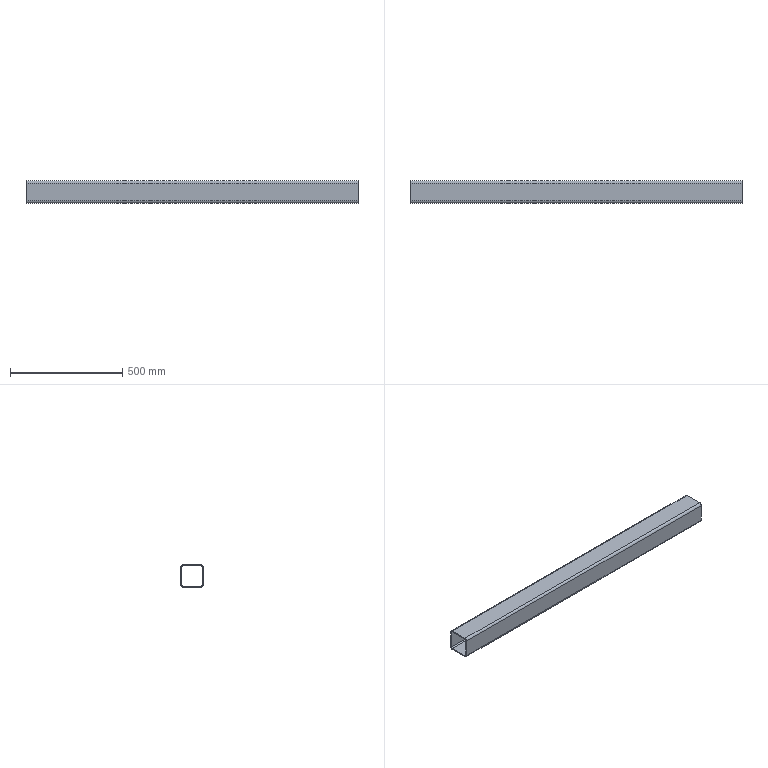Part | SolidWorks | features BaseBody 1 | 1 solid | 18 faces | box 1480 x 100 x 100 mm | volume 2716717 mm3 | plane 10 | cylinder 8 | commonest cylinder face diameters 10 x4 20 x4
STEP:
#1=CARTESIAN_POINT('',(-740.,40.,-50.));
#2=VERTEX_POINT('',#1);
#3=CARTESIAN_POINT('',(-740.,50.,-40.));
#4=VERTEX_POINT('',#3);
#5=CARTESIAN_POINT('',(-740.,40.,-40.));
#6=DIRECTION('',(1.,0.,0.));
#7=DIRECTION('',(0.,0.,-1.));
#8=AXIS2_PLACEMENT_3D('',#5,#6,#7);
#9=CIRCLE('',#8,10.);
#10=EDGE_CURVE('',#2,#4,#9,.T.);
#11=ORIENTED_EDGE('',*,*,#10,.T.);
#12=CARTESIAN_POINT('',(740.,50.,-40.));
#13=VERTEX_POINT('',#12);
#14=CARTESIAN_POINT('',(740.,50.,-40.));
#15=DIRECTION('',(-1.,0.,0.));
#16=VECTOR('',#15,1000.);
#17=LINE('',#14,#16);
#18=EDGE_CURVE('',#13,#4,#17,.T.);
#19=ORIENTED_EDGE('',*,*,#18,.F.);
#20=CARTESIAN_POINT('',(740.,40.,-50.));
#21=VERTEX_POINT('',#20);
#22=CARTESIAN_POINT('',(740.,40.,-40.));
#23=DIRECTION('',(1.,0.,0.));
#24=DIRECTION('',(0.,0.,-1.));
#25=AXIS2_PLACEMENT_3D('',#22,#23,#24);
#26=CIRCLE('',#25,10.);
#27=EDGE_CURVE('',#21,#13,#26,.T.);
#28=ORIENTED_EDGE('',*,*,#27,.F.);
#29=CARTESIAN_POINT('',(740.,40.,-50.));
#30=DIRECTION('',(-1.,0.,0.));
#31=VECTOR('',#30,1000.);
#32=LINE('',#29,#31);
#33=EDGE_CURVE('',#21,#2,#32,.T.);
#34=ORIENTED_EDGE('',*,*,#33,.T.);
#35=EDGE_LOOP('',(#11,#19,#28,#34));
#36=FACE_OUTER_BOUND('',#35,.T.);
#37=CARTESIAN_POINT('',(740.,40.,-40.));
#38=DIRECTION('',(-1.,0.,0.));
#39=DIRECTION('',(0.,0.,1.));
#40=AXIS2_PLACEMENT_3D('',#37,#38,#39);
#41=CYLINDRICAL_SURFACE('',#40,10.);
#42=ADVANCED_FACE('',(#36),#41,.T.);
#43=CARTESIAN_POINT('',(-740.,50.,40.));
#44=VERTEX_POINT('',#43);
#45=CARTESIAN_POINT('',(-740.,50.,-40.));
#46=DIRECTION('',(0.,0.,1.));
#47=VECTOR('',#46,1000.);
#48=LINE('',#45,#47);
#49=EDGE_CURVE('',#4,#44,#48,.T.);
#50=ORIENTED_EDGE('',*,*,#49,.T.);
#51=CARTESIAN_POINT('',(740.,50.,40.));
#52=VERTEX_POINT('',#51);
#53=CARTESIAN_POINT('',(740.,50.,40.));
#54=DIRECTION('',(-1.,0.,0.));
#55=VECTOR('',#54,1000.);
#56=LINE('',#53,#55);
#57=EDGE_CURVE('',#52,#44,#56,.T.);
#58=ORIENTED_EDGE('',*,*,#57,.F.);
#59=CARTESIAN_POINT('',(740.,50.,-40.));
#60=DIRECTION('',(0.,0.,1.));
#61=VECTOR('',#60,1000.);
#62=LINE('',#59,#61);
#63=EDGE_CURVE('',#13,#52,#62,.T.);
#64=ORIENTED_EDGE('',*,*,#63,.F.);
#65=ORIENTED_EDGE('',*,*,#18,.T.);
#66=EDGE_LOOP('',(#50,#58,#64,#65));
#67=FACE_OUTER_BOUND('',#66,.T.);
#68=CARTESIAN_POINT('',(740.,50.,-40.));
#69=DIRECTION('',(0.,-1.,0.));
#70=DIRECTION('',(0.,0.,-1.));
#71=AXIS2_PLACEMENT_3D('',#68,#69,#70);
#72=PLANE('',#71);
#73=ADVANCED_FACE('',(#67),#72,.F.);
#74=CARTESIAN_POINT('',(-740.,40.,50.));
#75=VERTEX_POINT('',#74);
#76=CARTESIAN_POINT('',(-740.,40.,40.));
#77=DIRECTION('',(1.,0.,0.));
#78=DIRECTION('',(0.,0.,-1.));
#79=AXIS2_PLACEMENT_3D('',#76,#77,#78);
#80=CIRCLE('',#79,10.);
#81=EDGE_CURVE('',#44,#75,#80,.T.);
#82=ORIENTED_EDGE('',*,*,#81,.T.);
#83=CARTESIAN_POINT('',(740.,40.,50.));
#84=VERTEX_POINT('',#83);
#85=CARTESIAN_POINT('',(740.,40.,50.));
#86=DIRECTION('',(-1.,0.,0.));
#87=VECTOR('',#86,1000.);
#88=LINE('',#85,#87);
#89=EDGE_CURVE('',#84,#75,#88,.T.);
#90=ORIENTED_EDGE('',*,*,#89,.F.);
#91=CARTESIAN_POINT('',(740.,40.,40.));
#92=DIRECTION('',(1.,0.,0.));
#93=DIRECTION('',(0.,0.,-1.));
#94=AXIS2_PLACEMENT_3D('',#91,#92,#93);
#95=CIRCLE('',#94,10.);
#96=EDGE_CURVE('',#52,#84,#95,.T.);
#97=ORIENTED_EDGE('',*,*,#96,.F.);
#98=ORIENTED_EDGE('',*,*,#57,.T.);
#99=EDGE_LOOP('',(#82,#90,#97,#98));
#100=FACE_OUTER_BOUND('',#99,.T.);
#101=CARTESIAN_POINT('',(740.,40.,40.));
#102=DIRECTION('',(-1.,0.,0.));
#103=DIRECTION('',(0.,0.,1.));
#104=AXIS2_PLACEMENT_3D('',#101,#102,#103);
#105=CYLINDRICAL_SURFACE('',#104,10.);
#106=ADVANCED_FACE('',(#100),#105,.T.);
#107=CARTESIAN_POINT('',(-740.,-40.,50.));
#108=VERTEX_POINT('',#107);
#109=CARTESIAN_POINT('',(-740.,-40.,50.));
#110=DIRECTION('',(0.,-1.,0.));
#111=VECTOR('',#110,1000.);
#112=LINE('',#109,#111);
#113=EDGE_CURVE('',#75,#108,#112,.T.);
#114=ORIENTED_EDGE('',*,*,#113,.T.);
#115=CARTESIAN_POINT('',(740.,-40.,50.));
#116=VERTEX_POINT('',#115);
#117=CARTESIAN_POINT('',(740.,-40.,50.));
#118=DIRECTION('',(-1.,0.,0.));
#119=VECTOR('',#118,1000.);
#120=LINE('',#117,#119);
#121=EDGE_CURVE('',#116,#108,#120,.T.);
#122=ORIENTED_EDGE('',*,*,#121,.F.);
#123=CARTESIAN_POINT('',(740.,-40.,50.));
#124=DIRECTION('',(0.,-1.,0.));
#125=VECTOR('',#124,1000.);
#126=LINE('',#123,#125);
#127=EDGE_CURVE('',#84,#116,#126,.T.);
#128=ORIENTED_EDGE('',*,*,#127,.F.);
#129=ORIENTED_EDGE('',*,*,#89,.T.);
#130=EDGE_LOOP('',(#114,#122,#128,#129));
#131=FACE_OUTER_BOUND('',#130,.T.);
#132=CARTESIAN_POINT('',(740.,-40.,50.));
#133=DIRECTION('',(0.,0.,-1.));
#134=DIRECTION('',(-1.,0.,0.));
#135=AXIS2_PLACEMENT_3D('',#132,#133,#134);
#136=PLANE('',#135);
#137=ADVANCED_FACE('',(#131),#136,.F.);
#138=CARTESIAN_POINT('',(-740.,-50.,40.));
#139=VERTEX_POINT('',#138);
#140=CARTESIAN_POINT('',(-740.,-40.,40.));
#141=DIRECTION('',(1.,0.,0.));
#142=DIRECTION('',(0.,0.,-1.));
#143=AXIS2_PLACEMENT_3D('',#140,#141,#142);
#144=CIRCLE('',#143,10.);
#145=EDGE_CURVE('',#108,#139,#144,.T.);
#146=ORIENTED_EDGE('',*,*,#145,.T.);
#147=CARTESIAN_POINT('',(740.,-50.,40.));
#148=VERTEX_POINT('',#147);
#149=CARTESIAN_POINT('',(740.,-50.,40.));
#150=DIRECTION('',(-1.,0.,0.));
#151=VECTOR('',#150,1000.);
#152=LINE('',#149,#151);
#153=EDGE_CURVE('',#148,#139,#152,.T.);
#154=ORIENTED_EDGE('',*,*,#153,.F.);
#155=CARTESIAN_POINT('',(740.,-40.,40.));
#156=DIRECTION('',(1.,0.,0.));
#157=DIRECTION('',(0.,0.,-1.));
#158=AXIS2_PLACEMENT_3D('',#155,#156,#157);
#159=CIRCLE('',#158,10.);
#160=EDGE_CURVE('',#116,#148,#159,.T.);
#161=ORIENTED_EDGE('',*,*,#160,.F.);
#162=ORIENTED_EDGE('',*,*,#121,.T.);
#163=EDGE_LOOP('',(#146,#154,#161,#162));
#164=FACE_OUTER_BOUND('',#163,.T.);
#165=CARTESIAN_POINT('',(740.,-40.,40.));
#166=DIRECTION('',(-1.,0.,0.));
#167=DIRECTION('',(0.,0.,1.));
#168=AXIS2_PLACEMENT_3D('',#165,#166,#167);
#169=CYLINDRICAL_SURFACE('',#168,10.);
#170=ADVANCED_FACE('',(#164),#169,.T.);
#171=CARTESIAN_POINT('',(-740.,-50.,-40.));
#172=VERTEX_POINT('',#171);
#173=CARTESIAN_POINT('',(-740.,-50.,40.));
#174=DIRECTION('',(0.,0.,-1.));
#175=VECTOR('',#174,1000.);
#176=LINE('',#173,#175);
#177=EDGE_CURVE('',#139,#172,#176,.T.);
#178=ORIENTED_EDGE('',*,*,#177,.T.);
#179=CARTESIAN_POINT('',(740.,-50.,-40.));
#180=VERTEX_POINT('',#179);
#181=CARTESIAN_POINT('',(740.,-50.,-40.));
#182=DIRECTION('',(-1.,0.,0.));
#183=VECTOR('',#182,1000.);
#184=LINE('',#181,#183);
#185=EDGE_CURVE('',#180,#172,#184,.T.);
#186=ORIENTED_EDGE('',*,*,#185,.F.);
#187=CARTESIAN_POINT('',(740.,-50.,40.));
#188=DIRECTION('',(0.,0.,-1.));
#189=VECTOR('',#188,1000.);
#190=LINE('',#187,#189);
#191=EDGE_CURVE('',#148,#180,#190,.T.);
#192=ORIENTED_EDGE('',*,*,#191,.F.);
#193=ORIENTED_EDGE('',*,*,#153,.T.);
#194=EDGE_LOOP('',(#178,#186,#192,#193));
#195=FACE_OUTER_BOUND('',#194,.T.);
#196=CARTESIAN_POINT('',(740.,-50.,40.));
#197=DIRECTION('',(0.,1.,0.));
#198=DIRECTION('',(0.,0.,1.));
#199=AXIS2_PLACEMENT_3D('',#196,#197,#198);
#200=PLANE('',#199);
#201=ADVANCED_FACE('',(#195),#200,.F.);
#202=CARTESIAN_POINT('',(-740.,-40.,-50.));
#203=VERTEX_POINT('',#202);
#204=CARTESIAN_POINT('',(-740.,-40.,-40.));
#205=DIRECTION('',(1.,0.,0.));
#206=DIRECTION('',(0.,0.,-1.));
#207=AXIS2_PLACEMENT_3D('',#204,#205,#206);
#208=CIRCLE('',#207,10.);
#209=EDGE_CURVE('',#172,#203,#208,.T.);
#210=ORIENTED_EDGE('',*,*,#209,.T.);
#211=CARTESIAN_POINT('',(740.,-40.,-50.));
#212=VERTEX_POINT('',#211);
#213=CARTESIAN_POINT('',(740.,-40.,-50.));
#214=DIRECTION('',(-1.,0.,0.));
#215=VECTOR('',#214,1000.);
#216=LINE('',#213,#215);
#217=EDGE_CURVE('',#212,#203,#216,.T.);
#218=ORIENTED_EDGE('',*,*,#217,.F.);
#219=CARTESIAN_POINT('',(740.,-40.,-40.));
#220=DIRECTION('',(1.,0.,0.));
#221=DIRECTION('',(0.,0.,-1.));
#222=AXIS2_PLACEMENT_3D('',#219,#220,#221);
#223=CIRCLE('',#222,10.);
#224=EDGE_CURVE('',#180,#212,#223,.T.);
#225=ORIENTED_EDGE('',*,*,#224,.F.);
#226=ORIENTED_EDGE('',*,*,#185,.T.);
#227=EDGE_LOOP('',(#210,#218,#225,#226));
#228=FACE_OUTER_BOUND('',#227,.T.);
#229=CARTESIAN_POINT('',(740.,-40.,-40.));
#230=DIRECTION('',(-1.,0.,0.));
#231=DIRECTION('',(0.,0.,1.));
#232=AXIS2_PLACEMENT_3D('',#229,#230,#231);
#233=CYLINDRICAL_SURFACE('',#232,10.);
#234=ADVANCED_FACE('',(#228),#233,.T.);
#235=CARTESIAN_POINT('',(-740.,45.,40.));
#236=VERTEX_POINT('',#235);
#237=CARTESIAN_POINT('',(-740.,40.,45.));
#238=VERTEX_POINT('',#237);
#239=CARTESIAN_POINT('',(-740.,40.,40.));
#240=DIRECTION('',(1.,0.,0.));
#241=DIRECTION('',(0.,0.,-1.));
#242=AXIS2_PLACEMENT_3D('',#239,#240,#241);
#243=CIRCLE('',#242,5.);
#244=EDGE_CURVE('',#236,#238,#243,.T.);
#245=ORIENTED_EDGE('',*,*,#244,.F.);
#246=CARTESIAN_POINT('',(740.,45.,40.));
#247=VERTEX_POINT('',#246);
#248=CARTESIAN_POINT('',(740.,45.,40.));
#249=DIRECTION('',(-1.,0.,0.));
#250=VECTOR('',#249,1000.);
#251=LINE('',#248,#250);
#252=EDGE_CURVE('',#247,#236,#251,.T.);
#253=ORIENTED_EDGE('',*,*,#252,.F.);
#254=CARTESIAN_POINT('',(740.,40.,45.));
#255=VERTEX_POINT('',#254);
#256=CARTESIAN_POINT('',(740.,40.,40.));
#257=DIRECTION('',(1.,0.,0.));
#258=DIRECTION('',(0.,0.,-1.));
#259=AXIS2_PLACEMENT_3D('',#256,#257,#258);
#260=CIRCLE('',#259,5.);
#261=EDGE_CURVE('',#247,#255,#260,.T.);
#262=ORIENTED_EDGE('',*,*,#261,.T.);
#263=CARTESIAN_POINT('',(740.,40.,45.));
#264=DIRECTION('',(-1.,0.,0.));
#265=VECTOR('',#264,1000.);
#266=LINE('',#263,#265);
#267=EDGE_CURVE('',#255,#238,#266,.T.);
#268=ORIENTED_EDGE('',*,*,#267,.T.);
#269=EDGE_LOOP('',(#245,#253,#262,#268));
#270=FACE_OUTER_BOUND('',#269,.T.);
#271=CARTESIAN_POINT('',(740.,40.,40.));
#272=DIRECTION('',(-1.,0.,0.));
#273=DIRECTION('',(0.,0.,1.));
#274=AXIS2_PLACEMENT_3D('',#271,#272,#273);
#275=CYLINDRICAL_SURFACE('',#274,5.);
#276=ADVANCED_FACE('',(#270),#275,.F.);
#277=CARTESIAN_POINT('',(-740.,45.,-40.));
#278=VERTEX_POINT('',#277);
#279=CARTESIAN_POINT('',(-740.,45.,-40.));
#280=DIRECTION('',(0.,0.,1.));
#281=VECTOR('',#280,1000.);
#282=LINE('',#279,#281);
#283=EDGE_CURVE('',#278,#236,#282,.T.);
#284=ORIENTED_EDGE('',*,*,#283,.F.);
#285=CARTESIAN_POINT('',(740.,45.,-40.));
#286=VERTEX_POINT('',#285);
#287=CARTESIAN_POINT('',(740.,45.,-40.));
#288=DIRECTION('',(-1.,0.,0.));
#289=VECTOR('',#288,1000.);
#290=LINE('',#287,#289);
#291=EDGE_CURVE('',#286,#278,#290,.T.);
#292=ORIENTED_EDGE('',*,*,#291,.F.);
#293=CARTESIAN_POINT('',(740.,45.,-40.));
#294=DIRECTION('',(0.,0.,1.));
#295=VECTOR('',#294,1000.);
#296=LINE('',#293,#295);
#297=EDGE_CURVE('',#286,#247,#296,.T.);
#298=ORIENTED_EDGE('',*,*,#297,.T.);
#299=ORIENTED_EDGE('',*,*,#252,.T.);
#300=EDGE_LOOP('',(#284,#292,#298,#299));
#301=FACE_OUTER_BOUND('',#300,.T.);
#302=CARTESIAN_POINT('',(740.,45.,-40.));
#303=DIRECTION('',(0.,-1.,0.));
#304=DIRECTION('',(0.,0.,-1.));
#305=AXIS2_PLACEMENT_3D('',#302,#303,#304);
#306=PLANE('',#305);
#307=ADVANCED_FACE('',(#301),#306,.T.);
#308=CARTESIAN_POINT('',(-740.,40.,-45.));
#309=VERTEX_POINT('',#308);
#310=CARTESIAN_POINT('',(-740.,40.,-40.));
#311=DIRECTION('',(1.,0.,0.));
#312=DIRECTION('',(0.,0.,-1.));
#313=AXIS2_PLACEMENT_3D('',#310,#311,#312);
#314=CIRCLE('',#313,5.);
#315=EDGE_CURVE('',#309,#278,#314,.T.);
#316=ORIENTED_EDGE('',*,*,#315,.F.);
#317=CARTESIAN_POINT('',(740.,40.,-45.));
#318=VERTEX_POINT('',#317);
#319=CARTESIAN_POINT('',(740.,40.,-45.));
#320=DIRECTION('',(-1.,0.,0.));
#321=VECTOR('',#320,1000.);
#322=LINE('',#319,#321);
#323=EDGE_CURVE('',#318,#309,#322,.T.);
#324=ORIENTED_EDGE('',*,*,#323,.F.);
#325=CARTESIAN_POINT('',(740.,40.,-40.));
#326=DIRECTION('',(1.,0.,0.));
#327=DIRECTION('',(0.,0.,-1.));
#328=AXIS2_PLACEMENT_3D('',#325,#326,#327);
#329=CIRCLE('',#328,5.);
#330=EDGE_CURVE('',#318,#286,#329,.T.);
#331=ORIENTED_EDGE('',*,*,#330,.T.);
#332=ORIENTED_EDGE('',*,*,#291,.T.);
#333=EDGE_LOOP('',(#316,#324,#331,#332));
#334=FACE_OUTER_BOUND('',#333,.T.);
#335=CARTESIAN_POINT('',(740.,40.,-40.));
#336=DIRECTION('',(-1.,0.,0.));
#337=DIRECTION('',(0.,0.,1.));
#338=AXIS2_PLACEMENT_3D('',#335,#336,#337);
#339=CYLINDRICAL_SURFACE('',#338,5.);
#340=ADVANCED_FACE('',(#334),#339,.F.);
#341=CARTESIAN_POINT('',(-740.,-40.,-45.));
#342=VERTEX_POINT('',#341);
#343=CARTESIAN_POINT('',(-740.,40.,-45.));
#344=DIRECTION('',(0.,1.,0.));
#345=VECTOR('',#344,1000.);
#346=LINE('',#343,#345);
#347=EDGE_CURVE('',#342,#309,#346,.T.);
#348=ORIENTED_EDGE('',*,*,#347,.F.);
#349=CARTESIAN_POINT('',(740.,-40.,-45.));
#350=VERTEX_POINT('',#349);
#351=CARTESIAN_POINT('',(740.,-40.,-45.));
#352=DIRECTION('',(-1.,0.,0.));
#353=VECTOR('',#352,1000.);
#354=LINE('',#351,#353);
#355=EDGE_CURVE('',#350,#342,#354,.T.);
#356=ORIENTED_EDGE('',*,*,#355,.F.);
#357=CARTESIAN_POINT('',(740.,40.,-45.));
#358=DIRECTION('',(0.,1.,0.));
#359=VECTOR('',#358,1000.);
#360=LINE('',#357,#359);
#361=EDGE_CURVE('',#350,#318,#360,.T.);
#362=ORIENTED_EDGE('',*,*,#361,.T.);
#363=ORIENTED_EDGE('',*,*,#323,.T.);
#364=EDGE_LOOP('',(#348,#356,#362,#363));
#365=FACE_OUTER_BOUND('',#364,.T.);
#366=CARTESIAN_POINT('',(740.,40.,-45.));
#367=DIRECTION('',(0.,0.,1.));
#368=DIRECTION('',(1.,0.,0.));
#369=AXIS2_PLACEMENT_3D('',#366,#367,#368);
#370=PLANE('',#369);
#371=ADVANCED_FACE('',(#365),#370,.T.);
#372=CARTESIAN_POINT('',(-740.,-45.,-40.));
#373=VERTEX_POINT('',#372);
#374=CARTESIAN_POINT('',(-740.,-40.,-40.));
#375=DIRECTION('',(1.,0.,0.));
#376=DIRECTION('',(0.,0.,-1.));
#377=AXIS2_PLACEMENT_3D('',#374,#375,#376);
#378=CIRCLE('',#377,5.);
#379=EDGE_CURVE('',#373,#342,#378,.T.);
#380=ORIENTED_EDGE('',*,*,#379,.F.);
#381=CARTESIAN_POINT('',(740.,-45.,-40.));
#382=VERTEX_POINT('',#381);
#383=CARTESIAN_POINT('',(740.,-45.,-40.));
#384=DIRECTION('',(-1.,0.,0.));
#385=VECTOR('',#384,1000.);
#386=LINE('',#383,#385);
#387=EDGE_CURVE('',#382,#373,#386,.T.);
#388=ORIENTED_EDGE('',*,*,#387,.F.);
#389=CARTESIAN_POINT('',(740.,-40.,-40.));
#390=DIRECTION('',(1.,0.,0.));
#391=DIRECTION('',(0.,0.,-1.));
#392=AXIS2_PLACEMENT_3D('',#389,#390,#391);
#393=CIRCLE('',#392,5.);
#394=EDGE_CURVE('',#382,#350,#393,.T.);
#395=ORIENTED_EDGE('',*,*,#394,.T.);
#396=ORIENTED_EDGE('',*,*,#355,.T.);
#397=EDGE_LOOP('',(#380,#388,#395,#396));
#398=FACE_OUTER_BOUND('',#397,.T.);
#399=CARTESIAN_POINT('',(740.,-40.,-40.));
#400=DIRECTION('',(-1.,0.,0.));
#401=DIRECTION('',(0.,0.,1.));
#402=AXIS2_PLACEMENT_3D('',#399,#400,#401);
#403=CYLINDRICAL_SURFACE('',#402,5.);
#404=ADVANCED_FACE('',(#398),#403,.F.);
#405=CARTESIAN_POINT('',(-740.,-45.,40.));
#406=VERTEX_POINT('',#405);
#407=CARTESIAN_POINT('',(-740.,-45.,40.));
#408=DIRECTION('',(0.,0.,-1.));
#409=VECTOR('',#408,1000.);
#410=LINE('',#407,#409);
#411=EDGE_CURVE('',#406,#373,#410,.T.);
#412=ORIENTED_EDGE('',*,*,#411,.F.);
#413=CARTESIAN_POINT('',(740.,-45.,40.));
#414=VERTEX_POINT('',#413);
#415=CARTESIAN_POINT('',(740.,-45.,40.));
#416=DIRECTION('',(-1.,0.,0.));
#417=VECTOR('',#416,1000.);
#418=LINE('',#415,#417);
#419=EDGE_CURVE('',#414,#406,#418,.T.);
#420=ORIENTED_EDGE('',*,*,#419,.F.);
#421=CARTESIAN_POINT('',(740.,-45.,40.));
#422=DIRECTION('',(0.,0.,-1.));
#423=VECTOR('',#422,1000.);
#424=LINE('',#421,#423);
#425=EDGE_CURVE('',#414,#382,#424,.T.);
#426=ORIENTED_EDGE('',*,*,#425,.T.);
#427=ORIENTED_EDGE('',*,*,#387,.T.);
#428=EDGE_LOOP('',(#412,#420,#426,#427));
#429=FACE_OUTER_BOUND('',#428,.T.);
#430=CARTESIAN_POINT('',(740.,-45.,40.));
#431=DIRECTION('',(0.,1.,0.));
#432=DIRECTION('',(0.,0.,1.));
#433=AXIS2_PLACEMENT_3D('',#430,#431,#432);
#434=PLANE('',#433);
#435=ADVANCED_FACE('',(#429),#434,.T.);
#436=CARTESIAN_POINT('',(-740.,-40.,45.));
#437=VERTEX_POINT('',#436);
#438=CARTESIAN_POINT('',(-740.,-40.,40.));
#439=DIRECTION('',(1.,0.,0.));
#440=DIRECTION('',(0.,0.,-1.));
#441=AXIS2_PLACEMENT_3D('',#438,#439,#440);
#442=CIRCLE('',#441,5.);
#443=EDGE_CURVE('',#437,#406,#442,.T.);
#444=ORIENTED_EDGE('',*,*,#443,.F.);
#445=CARTESIAN_POINT('',(740.,-40.,45.));
#446=VERTEX_POINT('',#445);
#447=CARTESIAN_POINT('',(740.,-40.,45.));
#448=DIRECTION('',(-1.,0.,0.));
#449=VECTOR('',#448,1000.);
#450=LINE('',#447,#449);
#451=EDGE_CURVE('',#446,#437,#450,.T.);
#452=ORIENTED_EDGE('',*,*,#451,.F.);
#453=CARTESIAN_POINT('',(740.,-40.,40.));
#454=DIRECTION('',(1.,0.,0.));
#455=DIRECTION('',(0.,0.,-1.));
#456=AXIS2_PLACEMENT_3D('',#453,#454,#455);
#457=CIRCLE('',#456,5.);
#458=EDGE_CURVE('',#446,#414,#457,.T.);
#459=ORIENTED_EDGE('',*,*,#458,.T.);
#460=ORIENTED_EDGE('',*,*,#419,.T.);
#461=EDGE_LOOP('',(#444,#452,#459,#460));
#462=FACE_OUTER_BOUND('',#461,.T.);
#463=CARTESIAN_POINT('',(740.,-40.,40.));
#464=DIRECTION('',(-1.,0.,0.));
#465=DIRECTION('',(0.,0.,1.));
#466=AXIS2_PLACEMENT_3D('',#463,#464,#465);
#467=CYLINDRICAL_SURFACE('',#466,5.);
#468=ADVANCED_FACE('',(#462),#467,.F.);
#469=CARTESIAN_POINT('',(-740.,-40.,45.));
#470=DIRECTION('',(0.,-1.,0.));
#471=VECTOR('',#470,1000.);
#472=LINE('',#469,#471);
#473=EDGE_CURVE('',#238,#437,#472,.T.);
#474=ORIENTED_EDGE('',*,*,#473,.F.);
#475=ORIENTED_EDGE('',*,*,#267,.F.);
#476=CARTESIAN_POINT('',(740.,-40.,45.));
#477=DIRECTION('',(0.,-1.,0.));
#478=VECTOR('',#477,1000.);
#479=LINE('',#476,#478);
#480=EDGE_CURVE('',#255,#446,#479,.T.);
#481=ORIENTED_EDGE('',*,*,#480,.T.);
#482=ORIENTED_EDGE('',*,*,#451,.T.);
#483=EDGE_LOOP('',(#474,#475,#481,#482));
#484=FACE_OUTER_BOUND('',#483,.T.);
#485=CARTESIAN_POINT('',(740.,-40.,45.));
#486=DIRECTION('',(0.,0.,-1.));
#487=DIRECTION('',(-1.,0.,0.));
#488=AXIS2_PLACEMENT_3D('',#485,#486,#487);
#489=PLANE('',#488);
#490=ADVANCED_FACE('',(#484),#489,.T.);
#491=CARTESIAN_POINT('',(-740.,40.,-50.));
#492=DIRECTION('',(0.,1.,0.));
#493=VECTOR('',#492,1000.);
#494=LINE('',#491,#493);
#495=EDGE_CURVE('',#203,#2,#494,.T.);
#496=ORIENTED_EDGE('',*,*,#495,.T.);
#497=ORIENTED_EDGE('',*,*,#33,.F.);
#498=CARTESIAN_POINT('',(740.,40.,-50.));
#499=DIRECTION('',(0.,1.,0.));
#500=VECTOR('',#499,1000.);
#501=LINE('',#498,#500);
#502=EDGE_CURVE('',#212,#21,#501,.T.);
#503=ORIENTED_EDGE('',*,*,#502,.F.);
#504=ORIENTED_EDGE('',*,*,#217,.T.);
#505=EDGE_LOOP('',(#496,#497,#503,#504));
#506=FACE_OUTER_BOUND('',#505,.T.);
#507=CARTESIAN_POINT('',(740.,40.,-50.));
#508=DIRECTION('',(0.,0.,1.));
#509=DIRECTION('',(1.,0.,0.));
#510=AXIS2_PLACEMENT_3D('',#507,#508,#509);
#511=PLANE('',#510);
#512=ADVANCED_FACE('',(#506),#511,.F.);
#513=ORIENTED_EDGE('',*,*,#261,.F.);
#514=ORIENTED_EDGE('',*,*,#297,.F.);
#515=ORIENTED_EDGE('',*,*,#330,.F.);
#516=ORIENTED_EDGE('',*,*,#361,.F.);
#517=ORIENTED_EDGE('',*,*,#394,.F.);
#518=ORIENTED_EDGE('',*,*,#425,.F.);
#519=ORIENTED_EDGE('',*,*,#458,.F.);
#520=ORIENTED_EDGE('',*,*,#480,.F.);
#521=EDGE_LOOP('',(#513,#514,#515,#516,#517,#518,#519,#520));
#522=FACE_BOUND('',#521,.T.);
#523=ORIENTED_EDGE('',*,*,#27,.T.);
#524=ORIENTED_EDGE('',*,*,#63,.T.);
#525=ORIENTED_EDGE('',*,*,#96,.T.);
#526=ORIENTED_EDGE('',*,*,#127,.T.);
#527=ORIENTED_EDGE('',*,*,#160,.T.);
#528=ORIENTED_EDGE('',*,*,#191,.T.);
#529=ORIENTED_EDGE('',*,*,#224,.T.);
#530=ORIENTED_EDGE('',*,*,#502,.T.);
#531=EDGE_LOOP('',(#523,#524,#525,#526,#527,#528,#529,#530));
#532=FACE_OUTER_BOUND('',#531,.T.);
#533=CARTESIAN_POINT('',(740.,40.,-40.));
#534=DIRECTION('',(1.,0.,0.));
#535=DIRECTION('',(0.,0.,-1.));
#536=AXIS2_PLACEMENT_3D('',#533,#534,#535);
#537=PLANE('',#536);
#538=ADVANCED_FACE('',(#522,#532),#537,.T.);
#539=ORIENTED_EDGE('',*,*,#244,.T.);
#540=ORIENTED_EDGE('',*,*,#473,.T.);
#541=ORIENTED_EDGE('',*,*,#443,.T.);
#542=ORIENTED_EDGE('',*,*,#411,.T.);
#543=ORIENTED_EDGE('',*,*,#379,.T.);
#544=ORIENTED_EDGE('',*,*,#347,.T.);
#545=ORIENTED_EDGE('',*,*,#315,.T.);
#546=ORIENTED_EDGE('',*,*,#283,.T.);
#547=EDGE_LOOP('',(#539,#540,#541,#542,#543,#544,#545,#546));
#548=FACE_BOUND('',#547,.T.);
#549=ORIENTED_EDGE('',*,*,#10,.F.);
#550=ORIENTED_EDGE('',*,*,#495,.F.);
#551=ORIENTED_EDGE('',*,*,#209,.F.);
#552=ORIENTED_EDGE('',*,*,#177,.F.);
#553=ORIENTED_EDGE('',*,*,#145,.F.);
#554=ORIENTED_EDGE('',*,*,#113,.F.);
#555=ORIENTED_EDGE('',*,*,#81,.F.);
#556=ORIENTED_EDGE('',*,*,#49,.F.);
#557=EDGE_LOOP('',(#549,#550,#551,#552,#553,#554,#555,#556));
#558=FACE_OUTER_BOUND('',#557,.T.);
#559=CARTESIAN_POINT('',(-740.,40.,-40.));
#560=DIRECTION('',(1.,0.,0.));
#561=DIRECTION('',(0.,0.,-1.));
#562=AXIS2_PLACEMENT_3D('',#559,#560,#561);
#563=PLANE('',#562);
#564=ADVANCED_FACE('',(#548,#558),#563,.F.);
#565=CLOSED_SHELL('',(#42,#73,#106,#137,#170,#201,#234,#276,#307,#340,#371,#404,#435,#468,#490,#512,#538,#564));
#566=MANIFOLD_SOLID_BREP('',#565);
#567=CARTESIAN_POINT('',(0.,0.,0.));
#568=DIRECTION('',(0.,0.,1.));
#569=DIRECTION('',(1.,0.,0.));
#570=AXIS2_PLACEMENT_3D('',#567,#568,#569);
#571=(LENGTH_UNIT()NAMED_UNIT(*)SI_UNIT(.MILLI.,.METRE.));
#572=UNCERTAINTY_MEASURE_WITH_UNIT(LENGTH_MEASURE(0.00001),#571,'','');
#573=(NAMED_UNIT(*)PLANE_ANGLE_UNIT()SI_UNIT($,.RADIAN.));
#574=(NAMED_UNIT(*)SI_UNIT($,.STERADIAN.)SOLID_ANGLE_UNIT());
#575=(GEOMETRIC_REPRESENTATION_CONTEXT(3)GLOBAL_UNCERTAINTY_ASSIGNED_CONTEXT((#572))GLOBAL_UNIT_ASSIGNED_CONTEXT((#571,#573,#574))REPRESENTATION_CONTEXT('',''));
#576=ADVANCED_BREP_SHAPE_REPRESENTATION('',(#566,#570),#575);